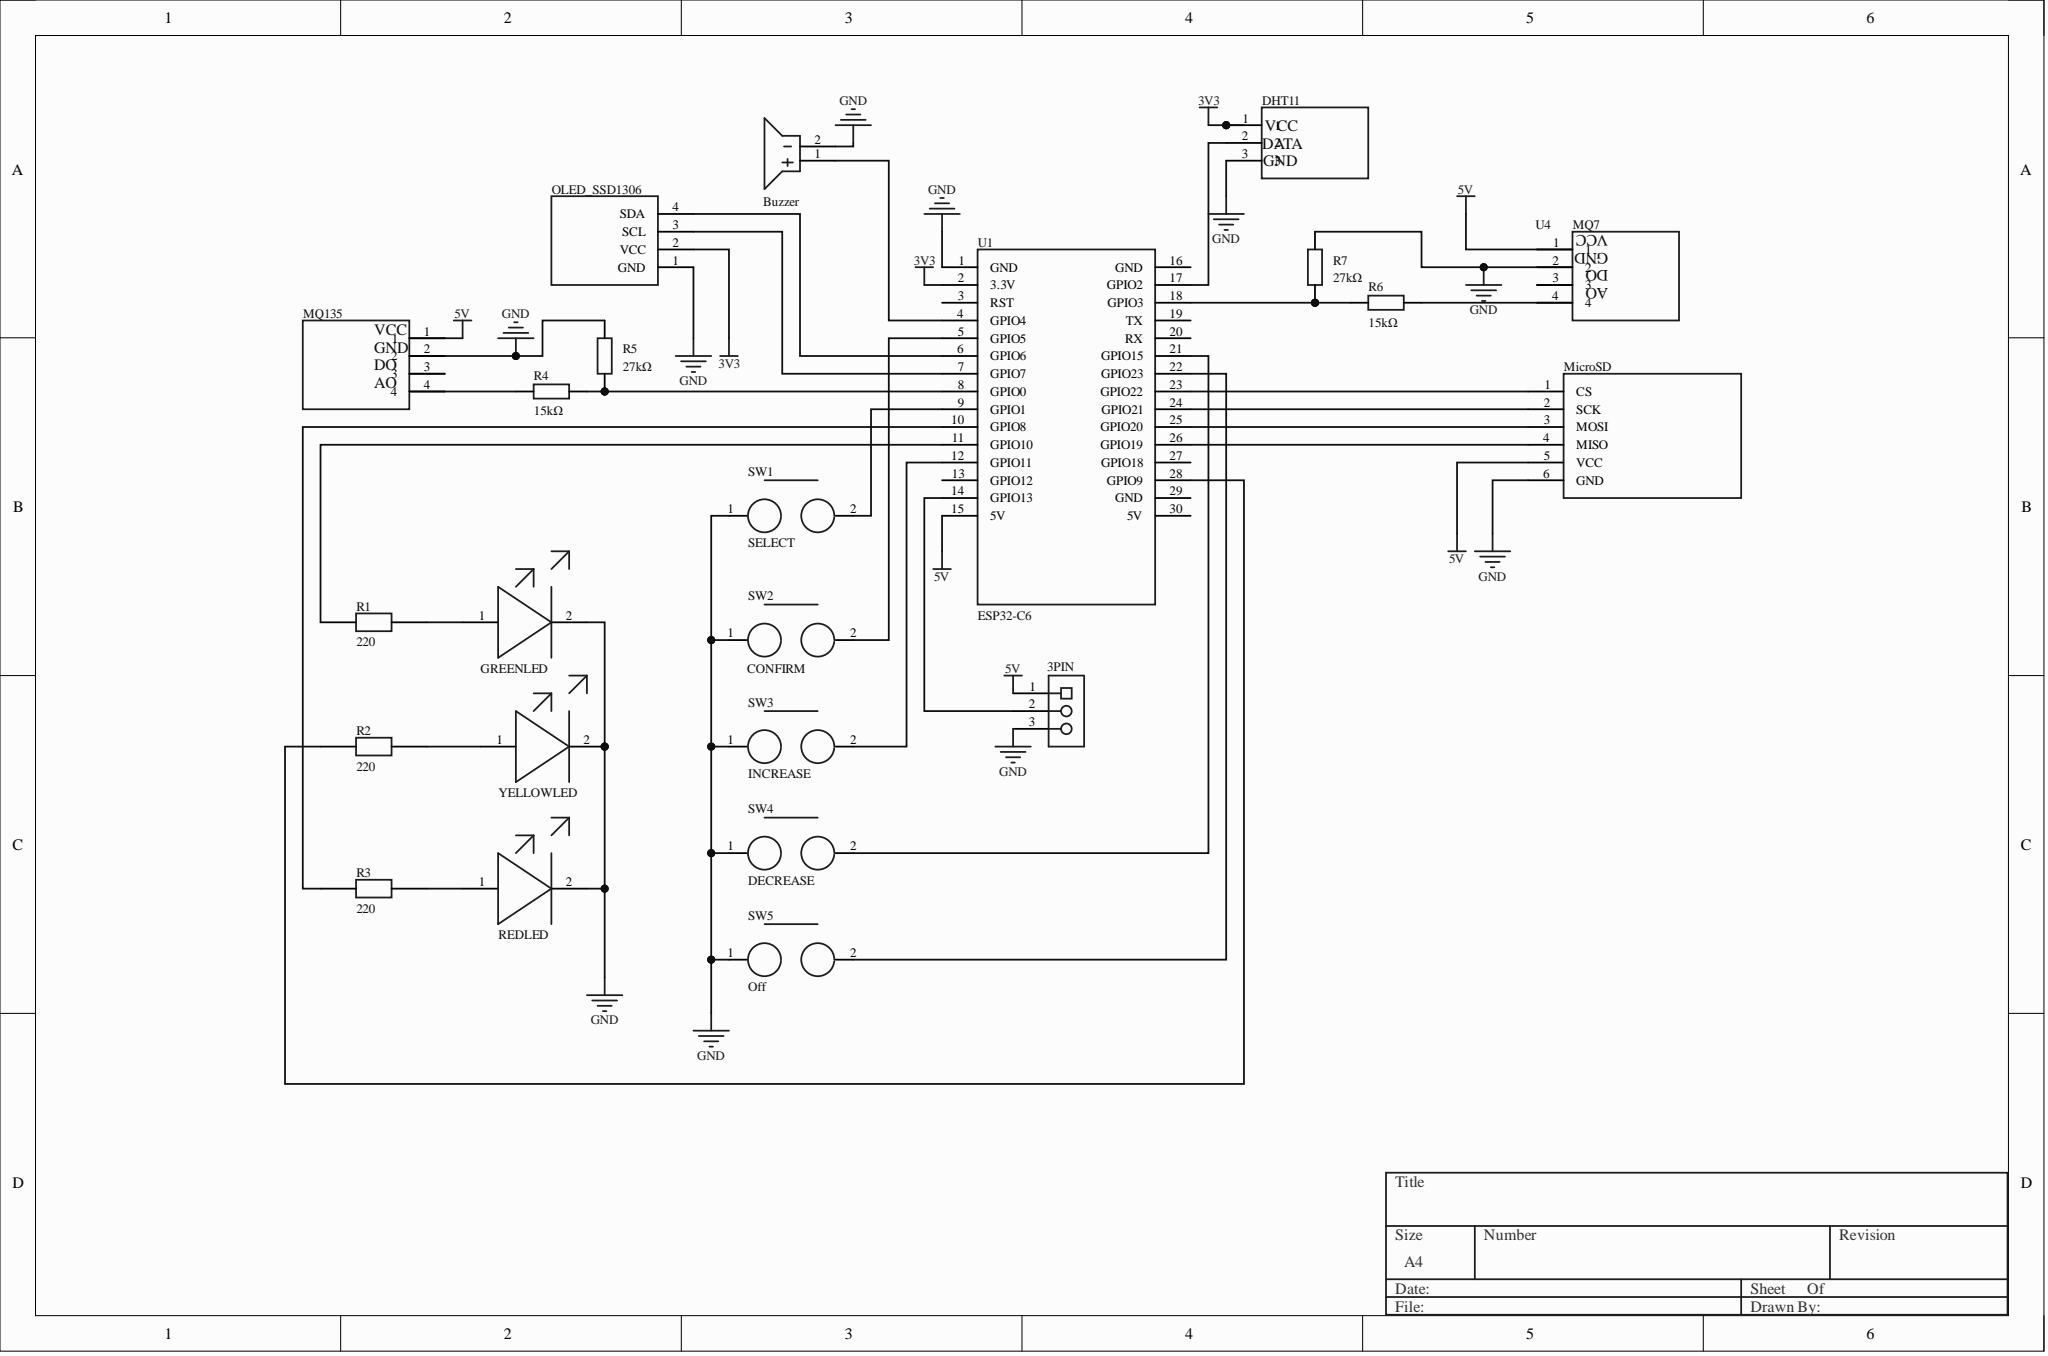Circuit board | Altium Designer | 23 parts | 27 nets
Bill of materials:
Comment,Description,Designator,Footprint,LibRef,Quantity
"DHT11","","","HDR-TH_3P-P2.54-V-F","DHT11","1"
"","Male Header, Pitch 2.5 mm, 1 x 3 Position, Height 6.1 mm, Tail Length 3.4 mm, -25 to 85 degC, RoHS, Bulk","3PIN","HDR-TH_3P-P2.54-V-F","CN-1P-M-R3","1"
"Buzzer","","Buzzer1","BUZ-TH_BD12.0-P6.00-D0.9-RD","Buzzer","1"
"LED_3M","","GREENLED, REDLED, YELLOWLED","LED_TH-3mm","LED_3M","3"
"220","","R1, R2, R3","Res_1/8W","220","3"
"15kΩ","","R4, R6","Res_1/8W","Res_AXIAL-1/8W","2"
"27kΩ","","R5, R7","Res_1/8W","Res_AXIAL-1/8W","2"
"SELECT","","SW1","KEY-TH_2P-L6.0-W6.0-P5.00","SELECT","1"
"CONFIRM","","SW2","KEY-TH_2P-L6.0-W6.0-P5.00","CONFIRM","1"
"INCREASE","","SW3","KEY-TH_2P-L6.0-W6.0-P5.00","INCREASE","1"
"DECREASE","","SW4","KEY-TH_2P-L6.0-W6.0-P5.00","DECREASE","1"
"Off","","SW5","KEY-TH_2P-L6.0-W6.0-P5.00","Off","1"
"ESP32-C6","","U1","HDR-TH_33P-P2.54-V-R2-C15-S2.54_C9041","ESP32-C6","1"
"MicroSD","","U2","HDR-TH_6P-P2.54-V-F","MicroSD","1"
"OLED_SSD1306","","U3","0.96OLED_4P","OLED_SSD1306","1"
"MQ7","","U4","HDR-TH_4P-P2.54-V-F","MQ7","1"
"MQ135","","U5","HDR-TH_4P-P2.54-V-F","MQ135","1"
Netlist (Protel format):
[
3PIN
HDR-TH_3P-P2.54-V-F




]
[
*
HDR-TH_3P-P2.54-V-F
DHT11



]
[
Buzzer1
BUZ-TH_BD12.0-P6.00-D0.9-RD
Buzzer



]
[
GREENLED
LED_TH-3mm
LED_3M



]
[
R1
Res_1/8W
220



]
[
R2
Res_1/8W
220



]
[
R3
Res_1/8W
220



]
[
R4
Res_1/8W
15kΩ



]
[
R5
Res_1/8W
27kΩ



]
[
R6
Res_1/8W
15kΩ



]
[
R7
Res_1/8W
27kΩ



]
[
REDLED
LED_TH-3mm
LED_3M



]
[
SW1
KEY-TH_2P-L6.0-W6.0-P5.00
SELECT



]
[
SW2
KEY-TH_2P-L6.0-W6.0-P5.00
CONFIRM



]
[
SW3
KEY-TH_2P-L6.0-W6.0-P5.00
INCREASE



]
[
SW4
KEY-TH_2P-L6.0-W6.0-P5.00
DECREASE



]
[
SW5
KEY-TH_2P-L6.0-W6.0-P5.00
Off



]
[
U1
HDR-TH_33P-P2.54-V-R2-C15-S2.54_C9041
ESP32-C6



]
[
U2
HDR-TH_6P-P2.54-V-F
MicroSD



]
[
U3
0.96OLED_4P
OLED_SSD1306



]
[
U4
HDR-TH_4P-P2.54-V-F
MQ7



]
[
U5
HDR-TH_4P-P2.54-V-F
MQ135



]
[
YELLOWLED
LED_TH-3mm
LED_3M



]
(
NetU1_26
U1-26
U2-4
)
(
NetU1_25
U1-25
U2-3
)
(
NetU1_24
U1-24
U2-2
)
(
NetU1_23
U1-23
U2-1
)
(
NetU1_7
U1-7
U3-3
)
(
NetU1_6
U1-6
U3-4
)
(
NetSW5_2
SW5-2
U1-22
)
(
NetSW4_2
SW4-2
U1-21
)
(
NetSW3_2
SW3-2
U1-12
)
(
NetSW2_2
SW2-2
U1-5
)
(
NetSW1_2
SW1-2
U1-9
)
(
NetR6_2
R6-2
U4-4
)
(
NetR6_1
R6-1
R7-1
U1-18
)
(
NetR4_2
R4-2
R5-1
U1-8
)
(
NetR4_1
R4-1
U5-4
)
(
NetR3_2
R3-2
REDLED-1
)
(
NetR3_1
R3-1
U1-10
)
(
NetR2_2
R2-2
YELLOWLED-1
)
(
NetR2_1
R2-1
U1-28
)
(
NetR1_1
R1-1
U1-11
)
(
NetGREENLED_1
GREENLED-1
R1-2
)
(
NetBuzzer1_1
Buzzer1-1
U1-4
)
(
Net*_2
*-2
U1-17
)
(
Net3PIN_2
3PIN-2
U1-14
)
(
GND
3PIN-3
*-3
Buzzer1-2
GREENLED-2
R5-2
R7-2
REDLED-2
SW1-1
SW2-1
SW3-1
SW4-1
SW5-1
U1-1
U2-6
U3-1
U4-2
U5-2
YELLOWLED-2
)
(
5V
3PIN-1
U1-15
U2-5
U4-1
U5-1
)
(
3V3
*-1
U1-2
U3-2
)